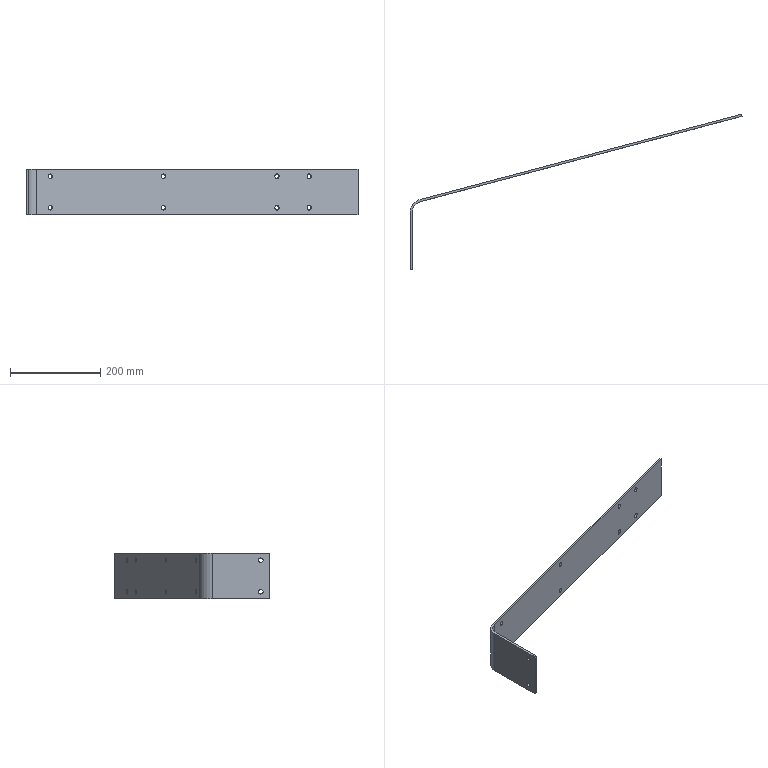Part | SolidWorks | features ICE 3, LPattern 3, ExtruThin 1 | 1 solid | 30 faces | box 736.282 x 345 x 100 mm | volume 446241 mm3 | cylinder 22 | plane 8 | commonest cylinder face diameters 10 x20 50 x1 60 x1
STEP:
#1=CARTESIAN_POINT('',(5.,20.,10.));
#2=VERTEX_POINT('',#1);
#3=CARTESIAN_POINT('',(5.,20.,20.));
#4=VERTEX_POINT('',#3);
#5=CARTESIAN_POINT('',(5.,20.,15.));
#6=DIRECTION('',(-1.,0.,0.));
#7=DIRECTION('',(0.,0.,1.));
#8=AXIS2_PLACEMENT_3D('',#5,#6,#7);
#9=CIRCLE('',#8,5.);
#10=EDGE_CURVE('',#2,#4,#9,.T.);
#11=ORIENTED_EDGE('',*,*,#10,.F.);
#12=CARTESIAN_POINT('',(0.,20.,10.));
#13=VERTEX_POINT('',#12);
#14=CARTESIAN_POINT('',(10.,20.,10.));
#15=DIRECTION('',(-1.,0.,0.));
#16=VECTOR('',#15,1000.);
#17=LINE('',#14,#16);
#18=EDGE_CURVE('',#2,#13,#17,.T.);
#19=ORIENTED_EDGE('',*,*,#18,.T.);
#20=CARTESIAN_POINT('',(0.,20.,20.));
#21=VERTEX_POINT('',#20);
#22=CARTESIAN_POINT('',(0.,20.,15.));
#23=DIRECTION('',(-1.,0.,0.));
#24=DIRECTION('',(0.,0.,1.));
#25=AXIS2_PLACEMENT_3D('',#22,#23,#24);
#26=CIRCLE('',#25,5.);
#27=EDGE_CURVE('',#13,#21,#26,.T.);
#28=ORIENTED_EDGE('',*,*,#27,.T.);
#29=CARTESIAN_POINT('',(10.,20.,20.));
#30=DIRECTION('',(-1.,0.,0.));
#31=VECTOR('',#30,1000.);
#32=LINE('',#29,#31);
#33=EDGE_CURVE('',#4,#21,#32,.T.);
#34=ORIENTED_EDGE('',*,*,#33,.F.);
#35=EDGE_LOOP('',(#11,#19,#28,#34));
#36=FACE_OUTER_BOUND('',#35,.T.);
#37=CARTESIAN_POINT('',(10.,20.,15.));
#38=DIRECTION('',(-1.,0.,0.));
#39=DIRECTION('',(0.,0.,1.));
#40=AXIS2_PLACEMENT_3D('',#37,#38,#39);
#41=CYLINDRICAL_SURFACE('',#40,5.);
#42=ADVANCED_FACE('',(#36),#41,.F.);
#43=CARTESIAN_POINT('',(5.,20.,80.));
#44=VERTEX_POINT('',#43);
#45=CARTESIAN_POINT('',(5.,20.,90.));
#46=VERTEX_POINT('',#45);
#47=CARTESIAN_POINT('',(5.,20.,85.));
#48=DIRECTION('',(-1.,0.,0.));
#49=DIRECTION('',(0.,0.,1.));
#50=AXIS2_PLACEMENT_3D('',#47,#48,#49);
#51=CIRCLE('',#50,5.);
#52=EDGE_CURVE('',#44,#46,#51,.T.);
#53=ORIENTED_EDGE('',*,*,#52,.F.);
#54=CARTESIAN_POINT('',(0.,20.,80.));
#55=VERTEX_POINT('',#54);
#56=CARTESIAN_POINT('',(10.,20.,80.));
#57=DIRECTION('',(-1.,0.,0.));
#58=VECTOR('',#57,1000.);
#59=LINE('',#56,#58);
#60=EDGE_CURVE('',#44,#55,#59,.T.);
#61=ORIENTED_EDGE('',*,*,#60,.T.);
#62=CARTESIAN_POINT('',(0.,20.,90.));
#63=VERTEX_POINT('',#62);
#64=CARTESIAN_POINT('',(0.,20.,85.));
#65=DIRECTION('',(-1.,0.,0.));
#66=DIRECTION('',(0.,0.,1.));
#67=AXIS2_PLACEMENT_3D('',#64,#65,#66);
#68=CIRCLE('',#67,5.);
#69=EDGE_CURVE('',#55,#63,#68,.T.);
#70=ORIENTED_EDGE('',*,*,#69,.T.);
#71=CARTESIAN_POINT('',(10.,20.,90.));
#72=DIRECTION('',(-1.,0.,0.));
#73=VECTOR('',#72,1000.);
#74=LINE('',#71,#73);
#75=EDGE_CURVE('',#46,#63,#74,.T.);
#76=ORIENTED_EDGE('',*,*,#75,.F.);
#77=EDGE_LOOP('',(#53,#61,#70,#76));
#78=FACE_OUTER_BOUND('',#77,.T.);
#79=CARTESIAN_POINT('',(10.,20.,85.));
#80=DIRECTION('',(-1.,0.,0.));
#81=DIRECTION('',(0.,0.,1.));
#82=AXIS2_PLACEMENT_3D('',#79,#80,#81);
#83=CYLINDRICAL_SURFACE('',#82,5.);
#84=ADVANCED_FACE('',(#78),#83,.F.);
#85=CARTESIAN_POINT('',(58.723,160.406,85.));
#86=VERTEX_POINT('',#85);
#87=CARTESIAN_POINT('',(49.057,157.842,85.));
#88=VERTEX_POINT('',#87);
#89=CARTESIAN_POINT('',(53.89,159.124,85.));
#90=DIRECTION('',(-0.2564,0.9666,0.));
#91=DIRECTION('',(-0.9666,-0.2564,0.));
#92=AXIS2_PLACEMENT_3D('',#89,#90,#91);
#93=CIRCLE('',#92,5.);
#94=EDGE_CURVE('',#86,#88,#93,.T.);
#95=ORIENTED_EDGE('',*,*,#94,.F.);
#96=CARTESIAN_POINT('',(57.44,165.239,85.));
#97=VERTEX_POINT('',#96);
#98=CARTESIAN_POINT('',(60.005,155.574,85.));
#99=DIRECTION('',(-0.2564,0.9666,0.));
#100=VECTOR('',#99,1000.);
#101=LINE('',#98,#100);
#102=EDGE_CURVE('',#86,#97,#101,.T.);
#103=ORIENTED_EDGE('',*,*,#102,.T.);
#104=CARTESIAN_POINT('',(47.775,162.675,85.));
#105=VERTEX_POINT('',#104);
#106=CARTESIAN_POINT('',(52.608,163.957,85.));
#107=DIRECTION('',(-0.2564,0.9666,0.));
#108=DIRECTION('',(-0.9666,-0.2564,0.));
#109=AXIS2_PLACEMENT_3D('',#106,#107,#108);
#110=CIRCLE('',#109,5.);
#111=EDGE_CURVE('',#97,#105,#110,.T.);
#112=ORIENTED_EDGE('',*,*,#111,.T.);
#113=CARTESIAN_POINT('',(50.339,153.009,85.));
#114=DIRECTION('',(-0.2564,0.9666,0.));
#115=VECTOR('',#114,1000.);
#116=LINE('',#113,#115);
#117=EDGE_CURVE('',#88,#105,#116,.T.);
#118=ORIENTED_EDGE('',*,*,#117,.F.);
#119=EDGE_LOOP('',(#95,#103,#112,#118));
#120=FACE_OUTER_BOUND('',#119,.T.);
#121=CARTESIAN_POINT('',(55.172,154.291,85.));
#122=DIRECTION('',(-0.2564,0.9666,0.));
#123=DIRECTION('',(-0.9666,-0.2564,0.));
#124=AXIS2_PLACEMENT_3D('',#121,#122,#123);
#125=CYLINDRICAL_SURFACE('',#124,5.);
#126=ADVANCED_FACE('',(#120),#125,.F.);
#127=CARTESIAN_POINT('',(310.029,227.079,85.));
#128=VERTEX_POINT('',#127);
#129=CARTESIAN_POINT('',(300.363,224.515,85.));
#130=VERTEX_POINT('',#129);
#131=CARTESIAN_POINT('',(305.196,225.797,85.));
#132=DIRECTION('',(-0.2564,0.9666,0.));
#133=DIRECTION('',(-0.9666,-0.2564,0.));
#134=AXIS2_PLACEMENT_3D('',#131,#132,#133);
#135=CIRCLE('',#134,5.);
#136=EDGE_CURVE('',#128,#130,#135,.T.);
#137=ORIENTED_EDGE('',*,*,#136,.F.);
#138=CARTESIAN_POINT('',(308.746,231.912,85.));
#139=VERTEX_POINT('',#138);
#140=CARTESIAN_POINT('',(311.311,222.247,85.));
#141=DIRECTION('',(-0.2564,0.9666,0.));
#142=VECTOR('',#141,1000.);
#143=LINE('',#140,#142);
#144=EDGE_CURVE('',#128,#139,#143,.T.);
#145=ORIENTED_EDGE('',*,*,#144,.T.);
#146=CARTESIAN_POINT('',(299.081,229.348,85.));
#147=VERTEX_POINT('',#146);
#148=CARTESIAN_POINT('',(303.914,230.63,85.));
#149=DIRECTION('',(-0.2564,0.9666,0.));
#150=DIRECTION('',(-0.9666,-0.2564,0.));
#151=AXIS2_PLACEMENT_3D('',#148,#149,#150);
#152=CIRCLE('',#151,5.);
#153=EDGE_CURVE('',#139,#147,#152,.T.);
#154=ORIENTED_EDGE('',*,*,#153,.T.);
#155=CARTESIAN_POINT('',(301.645,219.682,85.));
#156=DIRECTION('',(-0.2564,0.9666,0.));
#157=VECTOR('',#156,1000.);
#158=LINE('',#155,#157);
#159=EDGE_CURVE('',#130,#147,#158,.T.);
#160=ORIENTED_EDGE('',*,*,#159,.F.);
#161=EDGE_LOOP('',(#137,#145,#154,#160));
#162=FACE_OUTER_BOUND('',#161,.T.);
#163=CARTESIAN_POINT('',(306.478,220.965,85.));
#164=DIRECTION('',(-0.2564,0.9666,0.));
#165=DIRECTION('',(-0.9666,-0.2564,0.));
#166=AXIS2_PLACEMENT_3D('',#163,#164,#165);
#167=CYLINDRICAL_SURFACE('',#166,5.);
#168=ADVANCED_FACE('',(#162),#167,.F.);
#169=CARTESIAN_POINT('',(561.335,293.753,85.));
#170=VERTEX_POINT('',#169);
#171=CARTESIAN_POINT('',(551.669,291.188,85.));
#172=VERTEX_POINT('',#171);
#173=CARTESIAN_POINT('',(556.502,292.47,85.));
#174=DIRECTION('',(-0.2564,0.9666,0.));
#175=DIRECTION('',(-0.9666,-0.2564,0.));
#176=AXIS2_PLACEMENT_3D('',#173,#174,#175);
#177=CIRCLE('',#176,5.);
#178=EDGE_CURVE('',#170,#172,#177,.T.);
#179=ORIENTED_EDGE('',*,*,#178,.F.);
#180=CARTESIAN_POINT('',(560.052,298.585,85.));
#181=VERTEX_POINT('',#180);
#182=CARTESIAN_POINT('',(562.617,288.92,85.));
#183=DIRECTION('',(-0.2564,0.9666,0.));
#184=VECTOR('',#183,1000.);
#185=LINE('',#182,#184);
#186=EDGE_CURVE('',#170,#181,#185,.T.);
#187=ORIENTED_EDGE('',*,*,#186,.T.);
#188=CARTESIAN_POINT('',(550.387,296.021,85.));
#189=VERTEX_POINT('',#188);
#190=CARTESIAN_POINT('',(555.22,297.303,85.));
#191=DIRECTION('',(-0.2564,0.9666,0.));
#192=DIRECTION('',(-0.9666,-0.2564,0.));
#193=AXIS2_PLACEMENT_3D('',#190,#191,#192);
#194=CIRCLE('',#193,5.);
#195=EDGE_CURVE('',#181,#189,#194,.T.);
#196=ORIENTED_EDGE('',*,*,#195,.T.);
#197=CARTESIAN_POINT('',(552.951,286.355,85.));
#198=DIRECTION('',(-0.2564,0.9666,0.));
#199=VECTOR('',#198,1000.);
#200=LINE('',#197,#199);
#201=EDGE_CURVE('',#172,#189,#200,.T.);
#202=ORIENTED_EDGE('',*,*,#201,.F.);
#203=EDGE_LOOP('',(#179,#187,#196,#202));
#204=FACE_OUTER_BOUND('',#203,.T.);
#205=CARTESIAN_POINT('',(557.784,287.638,85.));
#206=DIRECTION('',(-0.2564,0.9666,0.));
#207=DIRECTION('',(-0.9666,-0.2564,0.));
#208=AXIS2_PLACEMENT_3D('',#205,#206,#207);
#209=CYLINDRICAL_SURFACE('',#208,5.);
#210=ADVANCED_FACE('',(#204),#209,.F.);
#211=CARTESIAN_POINT('',(58.723,160.406,15.));
#212=VERTEX_POINT('',#211);
#213=CARTESIAN_POINT('',(49.057,157.842,15.));
#214=VERTEX_POINT('',#213);
#215=CARTESIAN_POINT('',(53.89,159.124,15.));
#216=DIRECTION('',(-0.2564,0.9666,0.));
#217=DIRECTION('',(-0.9666,-0.2564,0.));
#218=AXIS2_PLACEMENT_3D('',#215,#216,#217);
#219=CIRCLE('',#218,5.);
#220=EDGE_CURVE('',#212,#214,#219,.T.);
#221=ORIENTED_EDGE('',*,*,#220,.F.);
#222=CARTESIAN_POINT('',(57.44,165.239,15.));
#223=VERTEX_POINT('',#222);
#224=CARTESIAN_POINT('',(60.005,155.574,15.));
#225=DIRECTION('',(-0.2564,0.9666,0.));
#226=VECTOR('',#225,1000.);
#227=LINE('',#224,#226);
#228=EDGE_CURVE('',#212,#223,#227,.T.);
#229=ORIENTED_EDGE('',*,*,#228,.T.);
#230=CARTESIAN_POINT('',(47.775,162.675,15.));
#231=VERTEX_POINT('',#230);
#232=CARTESIAN_POINT('',(52.608,163.957,15.));
#233=DIRECTION('',(-0.2564,0.9666,0.));
#234=DIRECTION('',(-0.9666,-0.2564,0.));
#235=AXIS2_PLACEMENT_3D('',#232,#233,#234);
#236=CIRCLE('',#235,5.);
#237=EDGE_CURVE('',#223,#231,#236,.T.);
#238=ORIENTED_EDGE('',*,*,#237,.T.);
#239=CARTESIAN_POINT('',(50.339,153.009,15.));
#240=DIRECTION('',(-0.2564,0.9666,0.));
#241=VECTOR('',#240,1000.);
#242=LINE('',#239,#241);
#243=EDGE_CURVE('',#214,#231,#242,.T.);
#244=ORIENTED_EDGE('',*,*,#243,.F.);
#245=EDGE_LOOP('',(#221,#229,#238,#244));
#246=FACE_OUTER_BOUND('',#245,.T.);
#247=CARTESIAN_POINT('',(55.172,154.291,15.));
#248=DIRECTION('',(-0.2564,0.9666,0.));
#249=DIRECTION('',(-0.9666,-0.2564,0.));
#250=AXIS2_PLACEMENT_3D('',#247,#248,#249);
#251=CYLINDRICAL_SURFACE('',#250,5.);
#252=ADVANCED_FACE('',(#246),#251,.F.);
#253=CARTESIAN_POINT('',(310.029,227.079,15.));
#254=VERTEX_POINT('',#253);
#255=CARTESIAN_POINT('',(300.363,224.515,15.));
#256=VERTEX_POINT('',#255);
#257=CARTESIAN_POINT('',(305.196,225.797,15.));
#258=DIRECTION('',(-0.2564,0.9666,0.));
#259=DIRECTION('',(-0.9666,-0.2564,0.));
#260=AXIS2_PLACEMENT_3D('',#257,#258,#259);
#261=CIRCLE('',#260,5.);
#262=EDGE_CURVE('',#254,#256,#261,.T.);
#263=ORIENTED_EDGE('',*,*,#262,.F.);
#264=CARTESIAN_POINT('',(308.746,231.912,15.));
#265=VERTEX_POINT('',#264);
#266=CARTESIAN_POINT('',(311.311,222.247,15.));
#267=DIRECTION('',(-0.2564,0.9666,0.));
#268=VECTOR('',#267,1000.);
#269=LINE('',#266,#268);
#270=EDGE_CURVE('',#254,#265,#269,.T.);
#271=ORIENTED_EDGE('',*,*,#270,.T.);
#272=CARTESIAN_POINT('',(299.081,229.348,15.));
#273=VERTEX_POINT('',#272);
#274=CARTESIAN_POINT('',(303.914,230.63,15.));
#275=DIRECTION('',(-0.2564,0.9666,0.));
#276=DIRECTION('',(-0.9666,-0.2564,0.));
#277=AXIS2_PLACEMENT_3D('',#274,#275,#276);
#278=CIRCLE('',#277,5.);
#279=EDGE_CURVE('',#265,#273,#278,.T.);
#280=ORIENTED_EDGE('',*,*,#279,.T.);
#281=CARTESIAN_POINT('',(301.645,219.682,15.));
#282=DIRECTION('',(-0.2564,0.9666,0.));
#283=VECTOR('',#282,1000.);
#284=LINE('',#281,#283);
#285=EDGE_CURVE('',#256,#273,#284,.T.);
#286=ORIENTED_EDGE('',*,*,#285,.F.);
#287=EDGE_LOOP('',(#263,#271,#280,#286));
#288=FACE_OUTER_BOUND('',#287,.T.);
#289=CARTESIAN_POINT('',(306.478,220.965,15.));
#290=DIRECTION('',(-0.2564,0.9666,0.));
#291=DIRECTION('',(-0.9666,-0.2564,0.));
#292=AXIS2_PLACEMENT_3D('',#289,#290,#291);
#293=CYLINDRICAL_SURFACE('',#292,5.);
#294=ADVANCED_FACE('',(#288),#293,.F.);
#295=CARTESIAN_POINT('',(561.335,293.753,15.));
#296=VERTEX_POINT('',#295);
#297=CARTESIAN_POINT('',(551.669,291.188,15.));
#298=VERTEX_POINT('',#297);
#299=CARTESIAN_POINT('',(556.502,292.47,15.));
#300=DIRECTION('',(-0.2564,0.9666,0.));
#301=DIRECTION('',(-0.9666,-0.2564,0.));
#302=AXIS2_PLACEMENT_3D('',#299,#300,#301);
#303=CIRCLE('',#302,5.);
#304=EDGE_CURVE('',#296,#298,#303,.T.);
#305=ORIENTED_EDGE('',*,*,#304,.F.);
#306=CARTESIAN_POINT('',(560.052,298.585,15.));
#307=VERTEX_POINT('',#306);
#308=CARTESIAN_POINT('',(562.617,288.92,15.));
#309=DIRECTION('',(-0.2564,0.9666,0.));
#310=VECTOR('',#309,1000.);
#311=LINE('',#308,#310);
#312=EDGE_CURVE('',#296,#307,#311,.T.);
#313=ORIENTED_EDGE('',*,*,#312,.T.);
#314=CARTESIAN_POINT('',(550.387,296.021,15.));
#315=VERTEX_POINT('',#314);
#316=CARTESIAN_POINT('',(555.22,297.303,15.));
#317=DIRECTION('',(-0.2564,0.9666,0.));
#318=DIRECTION('',(-0.9666,-0.2564,0.));
#319=AXIS2_PLACEMENT_3D('',#316,#317,#318);
#320=CIRCLE('',#319,5.);
#321=EDGE_CURVE('',#307,#315,#320,.T.);
#322=ORIENTED_EDGE('',*,*,#321,.T.);
#323=CARTESIAN_POINT('',(552.951,286.355,15.));
#324=DIRECTION('',(-0.2564,0.9666,0.));
#325=VECTOR('',#324,1000.);
#326=LINE('',#323,#325);
#327=EDGE_CURVE('',#298,#315,#326,.T.);
#328=ORIENTED_EDGE('',*,*,#327,.F.);
#329=EDGE_LOOP('',(#305,#313,#322,#328));
#330=FACE_OUTER_BOUND('',#329,.T.);
#331=CARTESIAN_POINT('',(557.784,287.638,15.));
#332=DIRECTION('',(-0.2564,0.9666,0.));
#333=DIRECTION('',(-0.9666,-0.2564,0.));
#334=AXIS2_PLACEMENT_3D('',#331,#332,#333);
#335=CYLINDRICAL_SURFACE('',#334,5.);
#336=ADVANCED_FACE('',(#330),#335,.F.);
#337=CARTESIAN_POINT('',(632.86,312.729,85.));
#338=VERTEX_POINT('',#337);
#339=CARTESIAN_POINT('',(623.194,310.164,85.));
#340=VERTEX_POINT('',#339);
#341=CARTESIAN_POINT('',(628.027,311.447,85.));
#342=DIRECTION('',(-0.2564,0.9666,0.));
#343=DIRECTION('',(-0.9666,-0.2564,0.));
#344=AXIS2_PLACEMENT_3D('',#341,#342,#343);
#345=CIRCLE('',#344,5.);
#346=EDGE_CURVE('',#338,#340,#345,.T.);
#347=ORIENTED_EDGE('',*,*,#346,.F.);
#348=CARTESIAN_POINT('',(631.578,317.561,85.));
#349=VERTEX_POINT('',#348);
#350=CARTESIAN_POINT('',(634.142,307.896,85.));
#351=DIRECTION('',(-0.2564,0.9666,0.));
#352=VECTOR('',#351,1000.);
#353=LINE('',#350,#352);
#354=EDGE_CURVE('',#338,#349,#353,.T.);
#355=ORIENTED_EDGE('',*,*,#354,.T.);
#356=CARTESIAN_POINT('',(621.912,314.997,85.));
#357=VERTEX_POINT('',#356);
#358=CARTESIAN_POINT('',(626.745,316.279,85.));
#359=DIRECTION('',(-0.2564,0.9666,0.));
#360=DIRECTION('',(-0.9666,-0.2564,0.));
#361=AXIS2_PLACEMENT_3D('',#358,#359,#360);
#362=CIRCLE('',#361,5.);
#363=EDGE_CURVE('',#349,#357,#362,.T.);
#364=ORIENTED_EDGE('',*,*,#363,.T.);
#365=CARTESIAN_POINT('',(624.477,305.332,85.));
#366=DIRECTION('',(-0.2564,0.9666,0.));
#367=VECTOR('',#366,1000.);
#368=LINE('',#365,#367);
#369=EDGE_CURVE('',#340,#357,#368,.T.);
#370=ORIENTED_EDGE('',*,*,#369,.F.);
#371=EDGE_LOOP('',(#347,#355,#364,#370));
#372=FACE_OUTER_BOUND('',#371,.T.);
#373=CARTESIAN_POINT('',(629.309,306.614,85.));
#374=DIRECTION('',(-0.2564,0.9666,0.));
#375=DIRECTION('',(-0.9666,-0.2564,0.));
#376=AXIS2_PLACEMENT_3D('',#373,#374,#375);
#377=CYLINDRICAL_SURFACE('',#376,5.);
#378=ADVANCED_FACE('',(#372),#377,.F.);
#379=CARTESIAN_POINT('',(632.86,312.729,15.));
#380=VERTEX_POINT('',#379);
#381=CARTESIAN_POINT('',(623.194,310.164,15.));
#382=VERTEX_POINT('',#381);
#383=CARTESIAN_POINT('',(628.027,311.447,15.));
#384=DIRECTION('',(-0.2564,0.9666,0.));
#385=DIRECTION('',(-0.9666,-0.2564,0.));
#386=AXIS2_PLACEMENT_3D('',#383,#384,#385);
#387=CIRCLE('',#386,5.);
#388=EDGE_CURVE('',#380,#382,#387,.T.);
#389=ORIENTED_EDGE('',*,*,#388,.F.);
#390=CARTESIAN_POINT('',(631.578,317.561,15.));
#391=VERTEX_POINT('',#390);
#392=CARTESIAN_POINT('',(634.142,307.896,15.));
#393=DIRECTION('',(-0.2564,0.9666,0.));
#394=VECTOR('',#393,1000.);
#395=LINE('',#392,#394);
#396=EDGE_CURVE('',#380,#391,#395,.T.);
#397=ORIENTED_EDGE('',*,*,#396,.T.);
#398=CARTESIAN_POINT('',(621.912,314.997,15.));
#399=VERTEX_POINT('',#398);
#400=CARTESIAN_POINT('',(626.745,316.279,15.));
#401=DIRECTION('',(-0.2564,0.9666,0.));
#402=DIRECTION('',(-0.9666,-0.2564,0.));
#403=AXIS2_PLACEMENT_3D('',#400,#401,#402);
#404=CIRCLE('',#403,5.);
#405=EDGE_CURVE('',#391,#399,#404,.T.);
#406=ORIENTED_EDGE('',*,*,#405,.T.);
#407=CARTESIAN_POINT('',(624.477,305.332,15.));
#408=DIRECTION('',(-0.2564,0.9666,0.));
#409=VECTOR('',#408,1000.);
#410=LINE('',#407,#409);
#411=EDGE_CURVE('',#382,#399,#410,.T.);
#412=ORIENTED_EDGE('',*,*,#411,.F.);
#413=EDGE_LOOP('',(#389,#397,#406,#412));
#414=FACE_OUTER_BOUND('',#413,.T.);
#415=CARTESIAN_POINT('',(629.309,306.614,15.));
#416=DIRECTION('',(-0.2564,0.9666,0.));
#417=DIRECTION('',(-0.9666,-0.2564,0.));
#418=AXIS2_PLACEMENT_3D('',#415,#416,#417);
#419=CYLINDRICAL_SURFACE('',#418,5.);
#420=ADVANCED_FACE('',(#414),#419,.F.);
#421=CARTESIAN_POINT('',(305.196,225.797,15.));
#422=DIRECTION('',(-0.2564,0.9666,0.));
#423=DIRECTION('',(-0.9666,-0.2564,0.));
#424=AXIS2_PLACEMENT_3D('',#421,#422,#423);
#425=CIRCLE('',#424,5.);
#426=EDGE_CURVE('',#256,#254,#425,.T.);
#427=ORIENTED_EDGE('',*,*,#426,.T.);
#428=ORIENTED_EDGE('',*,*,#262,.T.);
#429=EDGE_LOOP('',(#427,#428));
#430=FACE_BOUND('',#429,.T.);
#431=CARTESIAN_POINT('',(556.502,292.47,15.));
#432=DIRECTION('',(-0.2564,0.9666,0.));
#433=DIRECTION('',(-0.9666,-0.2564,0.));
#434=AXIS2_PLACEMENT_3D('',#431,#432,#433);
#435=CIRCLE('',#434,5.);
#436=EDGE_CURVE('',#298,#296,#435,.T.);
#437=ORIENTED_EDGE('',*,*,#436,.T.);
#438=ORIENTED_EDGE('',*,*,#304,.T.);
#439=EDGE_LOOP('',(#437,#438));
#440=FACE_BOUND('',#439,.T.);
#441=CARTESIAN_POINT('',(628.027,311.447,85.));
#442=DIRECTION('',(-0.2564,0.9666,0.));
#443=DIRECTION('',(-0.9666,-0.2564,0.));
#444=AXIS2_PLACEMENT_3D('',#441,#442,#443);
#445=CIRCLE('',#444,5.);
#446=EDGE_CURVE('',#340,#338,#445,.T.);
#447=ORIENTED_EDGE('',*,*,#446,.T.);
#448=ORIENTED_EDGE('',*,*,#346,.T.);
#449=EDGE_LOOP('',(#447,#448));
#450=FACE_BOUND('',#449,.T.);
#451=CARTESIAN_POINT('',(628.027,311.447,15.));
#452=DIRECTION('',(-0.2564,0.9666,0.));
#453=DIRECTION('',(-0.9666,-0.2564,0.));
#454=AXIS2_PLACEMENT_3D('',#451,#452,#453);
#455=CIRCLE('',#454,5.);
#456=EDGE_CURVE('',#382,#380,#455,.T.);
#457=ORIENTED_EDGE('',*,*,#456,.T.);
#458=ORIENTED_EDGE('',*,*,#388,.T.);
#459=EDGE_LOOP('',(#457,#458));
#460=FACE_BOUND('',#459,.T.);
#461=CARTESIAN_POINT('',(23.589,151.085,0.));
#462=VERTEX_POINT('',#461);
#463=CARTESIAN_POINT('',(736.282,340.167,0.));
#464=VERTEX_POINT('',#463);
#465=CARTESIAN_POINT('',(23.589,151.085,0.));
#466=DIRECTION('',(0.9666,0.2564,0.));
#467=VECTOR('',#466,1000.);
#468=LINE('',#465,#467);
#469=EDGE_CURVE('',#462,#464,#468,.T.);
#470=ORIENTED_EDGE('',*,*,#469,.T.);
#471=CARTESIAN_POINT('',(736.282,340.167,100.));
#472=VERTEX_POINT('',#471);
#473=CARTESIAN_POINT('',(736.282,340.167,100.));
#474=DIRECTION('',(0.,0.,-1.));
#475=VECTOR('',#474,1000.);
#476=LINE('',#473,#475);
#477=EDGE_CURVE('',#472,#464,#476,.T.);
#478=ORIENTED_EDGE('',*,*,#477,.F.);
#479=CARTESIAN_POINT('',(23.589,151.085,100.));
#480=VERTEX_POINT('',#479);
#481=CARTESIAN_POINT('',(23.589,151.085,100.));
#482=DIRECTION('',(0.9666,0.2564,0.));
#483=VECTOR('',#482,1000.);
#484=LINE('',#481,#483);
#485=EDGE_CURVE('',#480,#472,#484,.T.);
#486=ORIENTED_EDGE('',*,*,#485,.F.);
#487=CARTESIAN_POINT('',(23.589,151.085,100.));
#488=DIRECTION('',(0.,0.,-1.));
#489=VECTOR('',#488,1000.);
#490=LINE('',#487,#489);
#491=EDGE_CURVE('',#480,#462,#490,.T.);
#492=ORIENTED_EDGE('',*,*,#491,.T.);
#493=EDGE_LOOP('',(#470,#478,#486,#492));
#494=FACE_OUTER_BOUND('',#493,.T.);
#495=CARTESIAN_POINT('',(53.89,159.124,15.));
#496=DIRECTION('',(-0.2564,0.9666,0.));
#497=DIRECTION('',(-0.9666,-0.2564,0.));
#498=AXIS2_PLACEMENT_3D('',#495,#496,#497);
#499=CIRCLE('',#498,5.);
#500=EDGE_CURVE('',#214,#212,#499,.T.);
#501=ORIENTED_EDGE('',*,*,#500,.T.);
#502=ORIENTED_EDGE('',*,*,#220,.T.);
#503=EDGE_LOOP('',(#501,#502));
#504=FACE_BOUND('',#503,.T.);
#505=CARTESIAN_POINT('',(556.502,292.47,85.));
#506=DIRECTION('',(-0.2564,0.9666,0.));
#507=DIRECTION('',(-0.9666,-0.2564,0.));
#508=AXIS2_PLACEMENT_3D('',#505,#506,#507);
#509=CIRCLE('',#508,5.);
#510=EDGE_CURVE('',#172,#170,#509,.T.);
#511=ORIENTED_EDGE('',*,*,#510,.T.);
#512=ORIENTED_EDGE('',*,*,#178,.T.);
#513=EDGE_LOOP('',(#511,#512));
#514=FACE_BOUND('',#513,.T.);
#515=CARTESIAN_POINT('',(305.196,225.797,85.));
#516=DIRECTION('',(-0.2564,0.9666,0.));
#517=DIRECTION('',(-0.9666,-0.2564,0.));
#518=AXIS2_PLACEMENT_3D('',#515,#516,#517);
#519=CIRCLE('',#518,5.);
#520=EDGE_CURVE('',#130,#128,#519,.T.);
#521=ORIENTED_EDGE('',*,*,#520,.T.);
#522=ORIENTED_EDGE('',*,*,#136,.T.);
#523=EDGE_LOOP('',(#521,#522));
#524=FACE_BOUND('',#523,.T.);
#525=CARTESIAN_POINT('',(53.89,159.124,85.));
#526=DIRECTION('',(-0.2564,0.9666,0.));
#527=DIRECTION('',(-0.9666,-0.2564,0.));
#528=AXIS2_PLACEMENT_3D('',#525,#526,#527);
#529=CIRCLE('',#528,5.);
#530=EDGE_CURVE('',#88,#86,#529,.T.);
#531=ORIENTED_EDGE('',*,*,#530,.T.);
#532=ORIENTED_EDGE('',*,*,#94,.T.);
#533=EDGE_LOOP('',(#531,#532));
#534=FACE_BOUND('',#533,.T.);
#535=CARTESIAN_POINT('',(23.589,151.085,100.));
#536=DIRECTION('',(-0.2564,0.9666,0.));
#537=DIRECTION('',(-0.9666,-0.2564,0.));
#538=AXIS2_PLACEMENT_3D('',#535,#536,#537);
#539=PLANE('',#538);
#540=ADVANCED_FACE('',(#430,#440,#450,#460,#494,#504,#514,#524,#534),#539,.F.);
#541=CARTESIAN_POINT('',(735.,345.,0.));
#542=VERTEX_POINT('',#541);
#543=CARTESIAN_POINT('',(735.,345.,0.));
#544=DIRECTION('',(0.2564,-0.9666,0.));
#545=VECTOR('',#544,1000.);
#546=LINE('',#543,#545);
#547=EDGE_CURVE('',#542,#464,#546,.T.);
#548=ORIENTED_EDGE('',*,*,#547,.F.);
#549=CARTESIAN_POINT('',(735.,345.,100.));
#550=VERTEX_POINT('',#549);
#551=CARTESIAN_POINT('',(735.,345.,100.));
#552=DIRECTION('',(0.,0.,-1.));
#553=VECTOR('',#552,1000.);
#554=LINE('',#551,#553);
#555=EDGE_CURVE('',#550,#542,#554,.T.);
#556=ORIENTED_EDGE('',*,*,#555,.F.);
#557=CARTESIAN_POINT('',(735.,345.,100.));
#558=DIRECTION('',(0.2564,-0.9666,0.));
#559=VECTOR('',#558,1000.);
#560=LINE('',#557,#559);
#561=EDGE_CURVE('',#550,#472,#560,.T.);
#562=ORIENTED_EDGE('',*,*,#561,.T.);
#563=ORIENTED_EDGE('',*,*,#477,.T.);
#564=EDGE_LOOP('',(#548,#556,#562,#563));
#565=FACE_OUTER_BOUND('',#564,.T.);
#566=CARTESIAN_POINT('',(735.,345.,100.));
#567=DIRECTION('',(0.9666,0.2564,0.));
#568=DIRECTION('',(-0.2564,0.9666,0.));
#569=AXIS2_PLACEMENT_3D('',#566,#567,#568);
#570=PLANE('',#569);
#571=ADVANCED_FACE('',(#565),#570,.T.);
#572=CARTESIAN_POINT('',(303.914,230.63,15.));
#573=DIRECTION('',(-0.2564,0.9666,0.));
#574=DIRECTION('',(-0.9666,-0.2564,0.));
#575=AXIS2_PLACEMENT_3D('',#572,#573,#574);
#576=CIRCLE('',#575,5.);
#577=EDGE_CURVE('',#273,#265,#576,.T.);
#578=ORIENTED_EDGE('',*,*,#577,.F.);
#579=ORIENTED_EDGE('',*,*,#279,.F.);
#580=EDGE_LOOP('',(#578,#579));
#581=FACE_BOUND('',#580,.T.);
#582=CARTESIAN_POINT('',(555.22,297.303,15.));
#583=DIRECTION('',(-0.2564,0.9666,0.));
#584=DIRECTION('',(-0.9666,-0.2564,0.));
#585=AXIS2_PLACEMENT_3D('',#582,#583,#584);
#586=CIRCLE('',#585,5.);
#587=EDGE_CURVE('',#315,#307,#586,.T.);
#588=ORIENTED_EDGE('',*,*,#587,.F.);
#589=ORIENTED_EDGE('',*,*,#321,.F.);
#590=EDGE_LOOP('',(#588,#589));
#591=FACE_BOUND('',#590,.T.);
#592=CARTESIAN_POINT('',(626.745,316.279,85.));
#593=DIRECTION('',(-0.2564,0.9666,0.));
#594=DIRECTION('',(-0.9666,-0.2564,0.));
#595=AXIS2_PLACEMENT_3D('',#592,#593,#594);
#596=CIRCLE('',#595,5.);
#597=EDGE_CURVE('',#357,#349,#596,.T.);
#598=ORIENTED_EDGE('',*,*,#597,.F.);
#599=ORIENTED_EDGE('',*,*,#363,.F.);
#600=EDGE_LOOP('',(#598,#599));
#601=FACE_BOUND('',#600,.T.);
#602=CARTESIAN_POINT('',(626.745,316.279,15.));
#603=DIRECTION('',(-0.2564,0.9666,0.));
#604=DIRECTION('',(-0.9666,-0.2564,0.));
#605=AXIS2_PLACEMENT_3D('',#602,#603,#604);
#606=CIRCLE('',#605,5.);
#607=EDGE_CURVE('',#399,#391,#606,.T.);
#608=ORIENTED_EDGE('',*,*,#607,.F.);
#609=ORIENTED_EDGE('',*,*,#405,.F.);
#610=EDGE_LOOP('',(#608,#609));
#611=FACE_BOUND('',#610,.T.);
#612=CARTESIAN_POINT('',(22.307,155.918,0.));
#613=VERTEX_POINT('',#612);
#614=CARTESIAN_POINT('',(22.307,155.918,0.));
#615=DIRECTION('',(0.9666,0.2564,0.));
#616=VECTOR('',#615,1000.);
#617=LINE('',#614,#616);
#618=EDGE_CURVE('',#613,#542,#617,.T.);
#619=ORIENTED_EDGE('',*,*,#618,.F.);
#620=CARTESIAN_POINT('',(22.307,155.918,100.));
#621=VERTEX_POINT('',#620);
#622=CARTESIAN_POINT('',(22.307,155.918,100.));
#623=DIRECTION('',(0.,0.,-1.));
#624=VECTOR('',#623,1000.);
#625=LINE('',#622,#624);
#626=EDGE_CURVE('',#621,#613,#625,.T.);
#627=ORIENTED_EDGE('',*,*,#626,.F.);
#628=CARTESIAN_POINT('',(22.307,155.918,100.));
#629=DIRECTION('',(0.9666,0.2564,0.));
#630=VECTOR('',#629,1000.);
#631=LINE('',#628,#630);
#632=EDGE_CURVE('',#621,#550,#631,.T.);
#633=ORIENTED_EDGE('',*,*,#632,.T.);
#634=ORIENTED_EDGE('',*,*,#555,.T.);
#635=EDGE_LOOP('',(#619,#627,#633,#634));
#636=FACE_OUTER_BOUND('',#635,.T.);
#637=CARTESIAN_POINT('',(52.608,163.957,15.));
#638=DIRECTION('',(-0.2564,0.9666,0.));
#639=DIRECTION('',(-0.9666,-0.2564,0.));
#640=AXIS2_PLACEMENT_3D('',#637,#638,#639);
#641=CIRCLE('',#640,5.);
#642=EDGE_CURVE('',#231,#223,#641,.T.);
#643=ORIENTED_EDGE('',*,*,#642,.F.);
#644=ORIENTED_EDGE('',*,*,#237,.F.);
#645=EDGE_LOOP('',(#643,#644));
#646=FACE_BOUND('',#645,.T.);
#647=CARTESIAN_POINT('',(555.22,297.303,85.));
#648=DIRECTION('',(-0.2564,0.9666,0.));
#649=DIRECTION('',(-0.9666,-0.2564,0.));
#650=AXIS2_PLACEMENT_3D('',#647,#648,#649);
#651=CIRCLE('',#650,5.);
#652=EDGE_CURVE('',#189,#181,#651,.T.);
#653=ORIENTED_EDGE('',*,*,#652,.F.);
#654=ORIENTED_EDGE('',*,*,#195,.F.);
#655=EDGE_LOOP('',(#653,#654));
#656=FACE_BOUND('',#655,.T.);
#657=CARTESIAN_POINT('',(303.914,230.63,85.));
#658=DIRECTION('',(-0.2564,0.9666,0.));
#659=DIRECTION('',(-0.9666,-0.2564,0.));
#660=AXIS2_PLACEMENT_3D('',#657,#658,#659);
#661=CIRCLE('',#660,5.);
#662=EDGE_CURVE('',#147,#139,#661,.T.);
#663=ORIENTED_EDGE('',*,*,#662,.F.);
#664=ORIENTED_EDGE('',*,*,#153,.F.);
#665=EDGE_LOOP('',(#663,#664));
#666=FACE_BOUND('',#665,.T.);
#667=CARTESIAN_POINT('',(52.608,163.957,85.));
#668=DIRECTION('',(-0.2564,0.9666,0.));
#669=DIRECTION('',(-0.9666,-0.2564,0.));
#670=AXIS2_PLACEMENT_3D('',#667,#668,#669);
#671=CIRCLE('',#670,5.);
#672=EDGE_CURVE('',#105,#97,#671,.T.);
#673=ORIENTED_EDGE('',*,*,#672,.F.);
#674=ORIENTED_EDGE('',*,*,#111,.F.);
#675=EDGE_LOOP('',(#673,#674));
#676=FACE_BOUND('',#675,.T.);
#677=CARTESIAN_POINT('',(22.307,155.918,100.));
#678=DIRECTION('',(-0.2564,0.9666,0.));
#679=DIRECTION('',(-0.9666,-0.2564,0.));
#680=AXIS2_PLACEMENT_3D('',#677,#678,#679);
#681=PLANE('',#680);
#682=ADVANCED_FACE('',(#581,#591,#601,#611,#636,#646,#656,#666,#676),#681,.T.);
#683=CARTESIAN_POINT('',(0.,126.921,0.));
#684=VERTEX_POINT('',#683);
#685=CARTESIAN_POINT('',(30.,126.921,0.));
#686=DIRECTION('',(0.,0.,-1.));
#687=DIRECTION('',(-1.,0.,0.));
#688=AXIS2_PLACEMENT_3D('',#685,#686,#687);
#689=CIRCLE('',#688,30.);
#690=EDGE_CURVE('',#684,#613,#689,.T.);
#691=ORIENTED_EDGE('',*,*,#690,.F.);
#692=CARTESIAN_POINT('',(0.,126.921,100.));
#693=VERTEX_POINT('',#692);
#694=CARTESIAN_POINT('',(0.,126.921,100.));
#695=DIRECTION('',(0.,0.,-1.));
#696=VECTOR('',#695,1000.);
#697=LINE('',#694,#696);
#698=EDGE_CURVE('',#693,#684,#697,.T.);
#699=ORIENTED_EDGE('',*,*,#698,.F.);
#700=CARTESIAN_POINT('',(30.,126.921,100.));
#701=DIRECTION('',(0.,0.,-1.));
#702=DIRECTION('',(-1.,0.,0.));
#703=AXIS2_PLACEMENT_3D('',#700,#701,#702);
#704=CIRCLE('',#703,30.);
#705=EDGE_CURVE('',#693,#621,#704,.T.);
#706=ORIENTED_EDGE('',*,*,#705,.T.);
#707=ORIENTED_EDGE('',*,*,#626,.T.);
#708=EDGE_LOOP('',(#691,#699,#706,#707));
#709=FACE_OUTER_BOUND('',#708,.T.);
#710=CARTESIAN_POINT('',(30.,126.921,100.));
#711=DIRECTION('',(0.,0.,-1.));
#712=DIRECTION('',(-1.,0.,0.));
#713=AXIS2_PLACEMENT_3D('',#710,#711,#712);
#714=CYLINDRICAL_SURFACE('',#713,30.);
#715=ADVANCED_FACE('',(#709),#714,.T.);
#716=CARTESIAN_POINT('',(0.,20.,15.));
#717=DIRECTION('',(-1.,0.,0.));
#718=DIRECTION('',(0.,0.,1.));
#719=AXIS2_PLACEMENT_3D('',#716,#717,#718);
#720=CIRCLE('',#719,5.);
#721=EDGE_CURVE('',#21,#13,#720,.T.);
#722=ORIENTED_EDGE('',*,*,#721,.F.);
#723=ORIENTED_EDGE('',*,*,#27,.F.);
#724=EDGE_LOOP('',(#722,#723));
#725=FACE_BOUND('',#724,.T.);
#726=CARTESIAN_POINT('',(0.,20.,85.));
#727=DIRECTION('',(-1.,0.,0.));
#728=DIRECTION('',(0.,0.,1.));
#729=AXIS2_PLACEMENT_3D('',#726,#727,#728);
#730=CIRCLE('',#729,5.);
#731=EDGE_CURVE('',#63,#55,#730,.T.);
#732=ORIENTED_EDGE('',*,*,#731,.F.);
#733=ORIENTED_EDGE('',*,*,#69,.F.);
#734=EDGE_LOOP('',(#732,#733));
#735=FACE_BOUND('',#734,.T.);
#736=CARTESIAN_POINT('',(0.,0.,0.));
#737=VERTEX_POINT('',#736);
#738=CARTESIAN_POINT('',(0.,0.,0.));
#739=DIRECTION('',(0.,1.,0.));
#740=VECTOR('',#739,1000.);
#741=LINE('',#738,#740);
#742=EDGE_CURVE('',#737,#684,#741,.T.);
#743=ORIENTED_EDGE('',*,*,#742,.F.);
#744=CARTESIAN_POINT('',(0.,0.,100.));
#745=VERTEX_POINT('',#744);
#746=CARTESIAN_POINT('',(0.,0.,100.));
#747=DIRECTION('',(0.,0.,-1.));
#748=VECTOR('',#747,1000.);
#749=LINE('',#746,#748);
#750=EDGE_CURVE('',#745,#737,#749,.T.);
#751=ORIENTED_EDGE('',*,*,#750,.F.);
#752=CARTESIAN_POINT('',(0.,0.,100.));
#753=DIRECTION('',(0.,1.,0.));
#754=VECTOR('',#753,1000.);
#755=LINE('',#752,#754);
#756=EDGE_CURVE('',#745,#693,#755,.T.);
#757=ORIENTED_EDGE('',*,*,#756,.T.);
#758=ORIENTED_EDGE('',*,*,#698,.T.);
#759=EDGE_LOOP('',(#743,#751,#757,#758));
#760=FACE_OUTER_BOUND('',#759,.T.);
#761=CARTESIAN_POINT('',(0.,0.,100.));
#762=DIRECTION('',(-1.,0.,0.));
#763=DIRECTION('',(0.,0.,1.));
#764=AXIS2_PLACEMENT_3D('',#761,#762,#763);
#765=PLANE('',#764);
#766=ADVANCED_FACE('',(#725,#735,#760),#765,.T.);
#767=CARTESIAN_POINT('',(5.,0.,0.));
#768=VERTEX_POINT('',#767);
#769=CARTESIAN_POINT('',(5.,0.,0.));
#770=DIRECTION('',(-1.,0.,0.));
#771=VECTOR('',#770,1000.);
#772=LINE('',#769,#771);
#773=EDGE_CURVE('',#768,#737,#772,.T.);
#774=ORIENTED_EDGE('',*,*,#773,.F.);
#775=CARTESIAN_POINT('',(5.,0.,100.));
#776=VERTEX_POINT('',#775);
#777=CARTESIAN_POINT('',(5.,0.,100.));
#778=DIRECTION('',(0.,0.,-1.));
#779=VECTOR('',#778,1000.);
#780=LINE('',#777,#779);
#781=EDGE_CURVE('',#776,#768,#780,.T.);
#782=ORIENTED_EDGE('',*,*,#781,.F.);
#783=CARTESIAN_POINT('',(5.,0.,100.));
#784=DIRECTION('',(-1.,0.,0.));
#785=VECTOR('',#784,1000.);
#786=LINE('',#783,#785);
#787=EDGE_CURVE('',#776,#745,#786,.T.);
#788=ORIENTED_EDGE('',*,*,#787,.T.);
#789=ORIENTED_EDGE('',*,*,#750,.T.);
#790=EDGE_LOOP('',(#774,#782,#788,#789));
#791=FACE_OUTER_BOUND('',#790,.T.);
#792=CARTESIAN_POINT('',(5.,0.,100.));
#793=DIRECTION('',(0.,-1.,0.));
#794=DIRECTION('',(0.,0.,-1.));
#795=AXIS2_PLACEMENT_3D('',#792,#793,#794);
#796=PLANE('',#795);
#797=ADVANCED_FACE('',(#791),#796,.T.);
#798=CARTESIAN_POINT('',(5.,20.,15.));
#799=DIRECTION('',(-1.,0.,0.));
#800=DIRECTION('',(0.,0.,1.));
#801=AXIS2_PLACEMENT_3D('',#798,#799,#800);
#802=CIRCLE('',#801,5.);
#803=EDGE_CURVE('',#4,#2,#802,.T.);
#804=ORIENTED_EDGE('',*,*,#803,.T.);
#805=ORIENTED_EDGE('',*,*,#10,.T.);
#806=EDGE_LOOP('',(#804,#805));
#807=FACE_BOUND('',#806,.T.);
#808=CARTESIAN_POINT('',(5.,20.,85.));
#809=DIRECTION('',(-1.,0.,0.));
#810=DIRECTION('',(0.,0.,1.));
#811=AXIS2_PLACEMENT_3D('',#808,#809,#810);
#812=CIRCLE('',#811,5.);
#813=EDGE_CURVE('',#46,#44,#812,.T.);
#814=ORIENTED_EDGE('',*,*,#813,.T.);
#815=ORIENTED_EDGE('',*,*,#52,.T.);
#816=EDGE_LOOP('',(#814,#815));
#817=FACE_BOUND('',#816,.T.);
#818=CARTESIAN_POINT('',(5.,126.921,0.));
#819=VERTEX_POINT('',#818);
#820=CARTESIAN_POINT('',(5.,0.,0.));
#821=DIRECTION('',(0.,1.,0.));
#822=VECTOR('',#821,1000.);
#823=LINE('',#820,#822);
#824=EDGE_CURVE('',#768,#819,#823,.T.);
#825=ORIENTED_EDGE('',*,*,#824,.T.);
#826=CARTESIAN_POINT('',(5.,126.921,100.));
#827=VERTEX_POINT('',#826);
#828=CARTESIAN_POINT('',(5.,126.921,100.));
#829=DIRECTION('',(0.,0.,-1.));
#830=VECTOR('',#829,1000.);
#831=LINE('',#828,#830);
#832=EDGE_CURVE('',#827,#819,#831,.T.);
#833=ORIENTED_EDGE('',*,*,#832,.F.);
#834=CARTESIAN_POINT('',(5.,0.,100.));
#835=DIRECTION('',(0.,1.,0.));
#836=VECTOR('',#835,1000.);
#837=LINE('',#834,#836);
#838=EDGE_CURVE('',#776,#827,#837,.T.);
#839=ORIENTED_EDGE('',*,*,#838,.F.);
#840=ORIENTED_EDGE('',*,*,#781,.T.);
#841=EDGE_LOOP('',(#825,#833,#839,#840));
#842=FACE_OUTER_BOUND('',#841,.T.);
#843=CARTESIAN_POINT('',(5.,0.,100.));
#844=DIRECTION('',(-1.,0.,0.));
#845=DIRECTION('',(0.,0.,1.));
#846=AXIS2_PLACEMENT_3D('',#843,#844,#845);
#847=PLANE('',#846);
#848=ADVANCED_FACE('',(#807,#817,#842),#847,.F.);
#849=CARTESIAN_POINT('',(30.,126.921,0.));
#850=DIRECTION('',(0.,0.,-1.));
#851=DIRECTION('',(1.,0.,0.));
#852=AXIS2_PLACEMENT_3D('',#849,#850,#851);
#853=CIRCLE('',#852,25.);
#854=EDGE_CURVE('',#819,#462,#853,.T.);
#855=ORIENTED_EDGE('',*,*,#854,.T.);
#856=ORIENTED_EDGE('',*,*,#491,.F.);
#857=CARTESIAN_POINT('',(30.,126.921,100.));
#858=DIRECTION('',(0.,0.,-1.));
#859=DIRECTION('',(1.,0.,0.));
#860=AXIS2_PLACEMENT_3D('',#857,#858,#859);
#861=CIRCLE('',#860,25.);
#862=EDGE_CURVE('',#827,#480,#861,.T.);
#863=ORIENTED_EDGE('',*,*,#862,.F.);
#864=ORIENTED_EDGE('',*,*,#832,.T.);
#865=EDGE_LOOP('',(#855,#856,#863,#864));
#866=FACE_OUTER_BOUND('',#865,.T.);
#867=CARTESIAN_POINT('',(30.,126.921,100.));
#868=DIRECTION('',(0.,0.,-1.));
#869=DIRECTION('',(-1.,0.,0.));
#870=AXIS2_PLACEMENT_3D('',#867,#868,#869);
#871=CYLINDRICAL_SURFACE('',#870,25.);
#872=ADVANCED_FACE('',(#866),#871,.F.);
#873=ORIENTED_EDGE('',*,*,#485,.T.);
#874=ORIENTED_EDGE('',*,*,#561,.F.);
#875=ORIENTED_EDGE('',*,*,#632,.F.);
#876=ORIENTED_EDGE('',*,*,#705,.F.);
#877=ORIENTED_EDGE('',*,*,#756,.F.);
#878=ORIENTED_EDGE('',*,*,#787,.F.);
#879=ORIENTED_EDGE('',*,*,#838,.T.);
#880=ORIENTED_EDGE('',*,*,#862,.T.);
#881=EDGE_LOOP('',(#873,#874,#875,#876,#877,#878,#879,#880));
#882=FACE_OUTER_BOUND('',#881,.T.);
#883=CARTESIAN_POINT('',(30.,126.921,100.));
#884=DIRECTION('',(0.,0.,-1.));
#885=DIRECTION('',(-1.,0.,0.));
#886=AXIS2_PLACEMENT_3D('',#883,#884,#885);
#887=PLANE('',#886);
#888=ADVANCED_FACE('',(#882),#887,.F.);
#889=ORIENTED_EDGE('',*,*,#469,.F.);
#890=ORIENTED_EDGE('',*,*,#854,.F.);
#891=ORIENTED_EDGE('',*,*,#824,.F.);
#892=ORIENTED_EDGE('',*,*,#773,.T.);
#893=ORIENTED_EDGE('',*,*,#742,.T.);
#894=ORIENTED_EDGE('',*,*,#690,.T.);
#895=ORIENTED_EDGE('',*,*,#618,.T.);
#896=ORIENTED_EDGE('',*,*,#547,.T.);
#897=EDGE_LOOP('',(#889,#890,#891,#892,#893,#894,#895,#896));
#898=FACE_OUTER_BOUND('',#897,.T.);
#899=CARTESIAN_POINT('',(30.,126.921,0.));
#900=DIRECTION('',(0.,0.,-1.));
#901=DIRECTION('',(-1.,0.,0.));
#902=AXIS2_PLACEMENT_3D('',#899,#900,#901);
#903=PLANE('',#902);
#904=ADVANCED_FACE('',(#898),#903,.T.);
#905=ORIENTED_EDGE('',*,*,#396,.F.);
#906=ORIENTED_EDGE('',*,*,#456,.F.);
#907=ORIENTED_EDGE('',*,*,#411,.T.);
#908=ORIENTED_EDGE('',*,*,#607,.T.);
#909=EDGE_LOOP('',(#905,#906,#907,#908));
#910=FACE_OUTER_BOUND('',#909,.T.);
#911=CARTESIAN_POINT('',(629.309,306.614,15.));
#912=DIRECTION('',(-0.2564,0.9666,0.));
#913=DIRECTION('',(-0.9666,-0.2564,0.));
#914=AXIS2_PLACEMENT_3D('',#911,#912,#913);
#915=CYLINDRICAL_SURFACE('',#914,5.);
#916=ADVANCED_FACE('',(#910),#915,.F.);
#917=ORIENTED_EDGE('',*,*,#354,.F.);
#918=ORIENTED_EDGE('',*,*,#446,.F.);
#919=ORIENTED_EDGE('',*,*,#369,.T.);
#920=ORIENTED_EDGE('',*,*,#597,.T.);
#921=EDGE_LOOP('',(#917,#918,#919,#920));
#922=FACE_OUTER_BOUND('',#921,.T.);
#923=CARTESIAN_POINT('',(629.309,306.614,85.));
#924=DIRECTION('',(-0.2564,0.9666,0.));
#925=DIRECTION('',(-0.9666,-0.2564,0.));
#926=AXIS2_PLACEMENT_3D('',#923,#924,#925);
#927=CYLINDRICAL_SURFACE('',#926,5.);
#928=ADVANCED_FACE('',(#922),#927,.F.);
#929=ORIENTED_EDGE('',*,*,#312,.F.);
#930=ORIENTED_EDGE('',*,*,#436,.F.);
#931=ORIENTED_EDGE('',*,*,#327,.T.);
#932=ORIENTED_EDGE('',*,*,#587,.T.);
#933=EDGE_LOOP('',(#929,#930,#931,#932));
#934=FACE_OUTER_BOUND('',#933,.T.);
#935=CARTESIAN_POINT('',(557.784,287.638,15.));
#936=DIRECTION('',(-0.2564,0.9666,0.));
#937=DIRECTION('',(-0.9666,-0.2564,0.));
#938=AXIS2_PLACEMENT_3D('',#935,#936,#937);
#939=CYLINDRICAL_SURFACE('',#938,5.);
#940=ADVANCED_FACE('',(#934),#939,.F.);
#941=ORIENTED_EDGE('',*,*,#270,.F.);
#942=ORIENTED_EDGE('',*,*,#426,.F.);
#943=ORIENTED_EDGE('',*,*,#285,.T.);
#944=ORIENTED_EDGE('',*,*,#577,.T.);
#945=EDGE_LOOP('',(#941,#942,#943,#944));
#946=FACE_OUTER_BOUND('',#945,.T.);
#947=CARTESIAN_POINT('',(306.478,220.965,15.));
#948=DIRECTION('',(-0.2564,0.9666,0.));
#949=DIRECTION('',(-0.9666,-0.2564,0.));
#950=AXIS2_PLACEMENT_3D('',#947,#948,#949);
#951=CYLINDRICAL_SURFACE('',#950,5.);
#952=ADVANCED_FACE('',(#946),#951,.F.);
#953=ORIENTED_EDGE('',*,*,#228,.F.);
#954=ORIENTED_EDGE('',*,*,#500,.F.);
#955=ORIENTED_EDGE('',*,*,#243,.T.);
#956=ORIENTED_EDGE('',*,*,#642,.T.);
#957=EDGE_LOOP('',(#953,#954,#955,#956));
#958=FACE_OUTER_BOUND('',#957,.T.);
#959=CARTESIAN_POINT('',(55.172,154.291,15.));
#960=DIRECTION('',(-0.2564,0.9666,0.));
#961=DIRECTION('',(-0.9666,-0.2564,0.));
#962=AXIS2_PLACEMENT_3D('',#959,#960,#961);
#963=CYLINDRICAL_SURFACE('',#962,5.);
#964=ADVANCED_FACE('',(#958),#963,.F.);
#965=ORIENTED_EDGE('',*,*,#186,.F.);
#966=ORIENTED_EDGE('',*,*,#510,.F.);
#967=ORIENTED_EDGE('',*,*,#201,.T.);
#968=ORIENTED_EDGE('',*,*,#652,.T.);
#969=EDGE_LOOP('',(#965,#966,#967,#968));
#970=FACE_OUTER_BOUND('',#969,.T.);
#971=CARTESIAN_POINT('',(557.784,287.638,85.));
#972=DIRECTION('',(-0.2564,0.9666,0.));
#973=DIRECTION('',(-0.9666,-0.2564,0.));
#974=AXIS2_PLACEMENT_3D('',#971,#972,#973);
#975=CYLINDRICAL_SURFACE('',#974,5.);
#976=ADVANCED_FACE('',(#970),#975,.F.);
#977=ORIENTED_EDGE('',*,*,#144,.F.);
#978=ORIENTED_EDGE('',*,*,#520,.F.);
#979=ORIENTED_EDGE('',*,*,#159,.T.);
#980=ORIENTED_EDGE('',*,*,#662,.T.);
#981=EDGE_LOOP('',(#977,#978,#979,#980));
#982=FACE_OUTER_BOUND('',#981,.T.);
#983=CARTESIAN_POINT('',(306.478,220.965,85.));
#984=DIRECTION('',(-0.2564,0.9666,0.));
#985=DIRECTION('',(-0.9666,-0.2564,0.));
#986=AXIS2_PLACEMENT_3D('',#983,#984,#985);
#987=CYLINDRICAL_SURFACE('',#986,5.);
#988=ADVANCED_FACE('',(#982),#987,.F.);
#989=ORIENTED_EDGE('',*,*,#102,.F.);
#990=ORIENTED_EDGE('',*,*,#530,.F.);
#991=ORIENTED_EDGE('',*,*,#117,.T.);
#992=ORIENTED_EDGE('',*,*,#672,.T.);
#993=EDGE_LOOP('',(#989,#990,#991,#992));
#994=FACE_OUTER_BOUND('',#993,.T.);
#995=CARTESIAN_POINT('',(55.172,154.291,85.));
#996=DIRECTION('',(-0.2564,0.9666,0.));
#997=DIRECTION('',(-0.9666,-0.2564,0.));
#998=AXIS2_PLACEMENT_3D('',#995,#996,#997);
#999=CYLINDRICAL_SURFACE('',#998,5.);
#1000=ADVANCED_FACE('',(#994),#999,.F.);
#1001=ORIENTED_EDGE('',*,*,#60,.F.);
#1002=ORIENTED_EDGE('',*,*,#813,.F.);
#1003=ORIENTED_EDGE('',*,*,#75,.T.);
#1004=ORIENTED_EDGE('',*,*,#731,.T.);
#1005=EDGE_LOOP('',(#1001,#1002,#1003,#1004));
#1006=FACE_OUTER_BOUND('',#1005,.T.);
#1007=CARTESIAN_POINT('',(10.,20.,85.));
#1008=DIRECTION('',(-1.,0.,0.));
#1009=DIRECTION('',(0.,0.,1.));
#1010=AXIS2_PLACEMENT_3D('',#1007,#1008,#1009);
#1011=CYLINDRICAL_SURFACE('',#1010,5.);
#1012=ADVANCED_FACE('',(#1006),#1011,.F.);
#1013=ORIENTED_EDGE('',*,*,#18,.F.);
#1014=ORIENTED_EDGE('',*,*,#803,.F.);
#1015=ORIENTED_EDGE('',*,*,#33,.T.);
#1016=ORIENTED_EDGE('',*,*,#721,.T.);
#1017=EDGE_LOOP('',(#1013,#1014,#1015,#1016));
#1018=FACE_OUTER_BOUND('',#1017,.T.);
#1019=CARTESIAN_POINT('',(10.,20.,15.));
#1020=DIRECTION('',(-1.,0.,0.));
#1021=DIRECTION('',(0.,0.,1.));
#1022=AXIS2_PLACEMENT_3D('',#1019,#1020,#1021);
#1023=CYLINDRICAL_SURFACE('',#1022,5.);
#1024=ADVANCED_FACE('',(#1018),#1023,.F.);
#1025=CLOSED_SHELL('',(#42,#84,#126,#168,#210,#252,#294,#336,#378,#420,#540,#571,#682,#715,#766,#797,#848,#872,#888,#904,#916,#928,#940,#952,#964,#976,#988,#1000,#1012,#1024));
#1026=MANIFOLD_SOLID_BREP('',#1025);
#1027=CARTESIAN_POINT('',(0.,0.,0.));
#1028=DIRECTION('',(0.,0.,1.));
#1029=DIRECTION('',(1.,0.,0.));
#1030=AXIS2_PLACEMENT_3D('',#1027,#1028,#1029);
#1031=(LENGTH_UNIT()NAMED_UNIT(*)SI_UNIT(.MILLI.,.METRE.));
#1032=UNCERTAINTY_MEASURE_WITH_UNIT(LENGTH_MEASURE(0.00001),#1031,'','');
#1033=(NAMED_UNIT(*)PLANE_ANGLE_UNIT()SI_UNIT($,.RADIAN.));
#1034=(NAMED_UNIT(*)SI_UNIT($,.STERADIAN.)SOLID_ANGLE_UNIT());
#1035=(GEOMETRIC_REPRESENTATION_CONTEXT(3)GLOBAL_UNCERTAINTY_ASSIGNED_CONTEXT((#1032))GLOBAL_UNIT_ASSIGNED_CONTEXT((#1031,#1033,#1034))REPRESENTATION_CONTEXT('',''));
#1036=ADVANCED_BREP_SHAPE_REPRESENTATION('',(#1026,#1030),#1035);